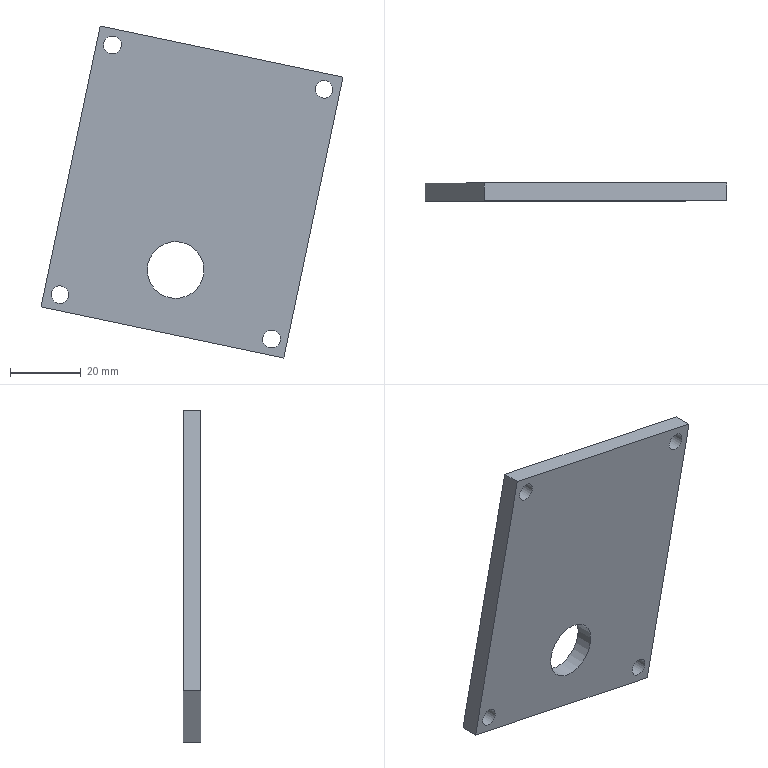Part | STEP file | 2_ESTAGIO_006-01 | 1 solid | 11 faces | box 85.161 x 5 x 93.664 mm | volume 26952 mm3 | plane 6 | cylinder 5 | commonest cylinder face diameters 5 x4 16 x1
STEP:
#1=CARTESIAN_POINT('',(0.,0.,0.));
#2=DIRECTION('',(0.,0.,1.));
#3=DIRECTION('',(1.,0.,0.));
#4=AXIS2_PLACEMENT_3D('',#1,#2,#3);
#5=CARTESIAN_POINT('',(432.411,-532.65,430.025));
#6=VERTEX_POINT('',#5);
#7=CARTESIAN_POINT('',(430.217,-532.65,428.827));
#8=DIRECTION('',(0.,-1.,0.));
#9=DIRECTION('',(1.,0.,0.));
#10=AXIS2_PLACEMENT_3D('',#7,#8,#9);
#11=CIRCLE('',#10,2.5);
#12=CARTESIAN_POINT('',(430.217,-532.75,428.827));
#13=DIRECTION('',(0.,-1.,0.));
#14=DIRECTION('',(0.8776,0.,0.4794));
#15=AXIS2_PLACEMENT_3D('',#12,#13,#14);
#16=CYLINDRICAL_SURFACE('',#15,2.5);
#17=CARTESIAN_POINT('',(-0.5,-0.1));
#18=DIRECTION('',(1.,0.));
#19=VECTOR('',#18,1.);
#20=LINE('',#17,#19);
#21=(GEOMETRIC_REPRESENTATION_CONTEXT(2)PARAMETRIC_REPRESENTATION_CONTEXT()REPRESENTATION_CONTEXT('',''));
#22=DEFINITIONAL_REPRESENTATION('',(#20),#21);
#23=PCURVE('',#16,#22);
#24=CARTESIAN_POINT('',(435.546,-532.65,432.305));
#25=DIRECTION('',(0.,1.,0.));
#26=DIRECTION('',(0.,0.,1.));
#27=AXIS2_PLACEMENT_3D('',#24,#25,#26);
#28=PLANE('',#27);
#29=CARTESIAN_POINT('',(-3.478,-2.829));
#30=CARTESIAN_POINT('',(0.8517,-2.829));
#31=CARTESIAN_POINT('',(-1.313,-6.579));
#32=CARTESIAN_POINT('',(-3.478,-10.329));
#33=CARTESIAN_POINT('',(-5.643,-6.579));
#34=CARTESIAN_POINT('',(-7.809,-2.829));
#35=CARTESIAN_POINT('',(-3.478,-2.829));
#36=(BOUNDED_CURVE()B_SPLINE_CURVE(2,(#29,#30,#31,#32,#33,#34,#35),.UNSPECIFIED.,.T.,.F.)B_SPLINE_CURVE_WITH_KNOTS((1,2,2,2,2,1),(-2.094,0.,2.094,4.189,6.283,8.378),.UNSPECIFIED.)CURVE()GEOMETRIC_REPRESENTATION_ITEM()RATIONAL_B_SPLINE_CURVE((1.,0.5,1.,0.5,1.,0.5,1.))REPRESENTATION_ITEM(''));
#37=(GEOMETRIC_REPRESENTATION_CONTEXT(2)PARAMETRIC_REPRESENTATION_CONTEXT()REPRESENTATION_CONTEXT('',''));
#38=DEFINITIONAL_REPRESENTATION('',(#36),#37);
#39=PCURVE('',#28,#38);
#40=SURFACE_CURVE('',#11,(#23,#39),.PCURVE_S1.);
#41=EDGE_CURVE('',#6,#6,#40,.T.);
#42=ORIENTED_EDGE('',*,*,#41,.T.);
#43=CARTESIAN_POINT('',(432.411,-537.65,430.025));
#44=VERTEX_POINT('',#43);
#45=CARTESIAN_POINT('',(432.411,-532.65,430.025));
#46=CARTESIAN_POINT('',(432.411,-537.65,430.025));
#47=B_SPLINE_CURVE_WITH_KNOTS('',1,(#45,#46),.UNSPECIFIED.,.F.,.F.,(2,2),(-0.1,4.9),.PIECEWISE_BEZIER_KNOTS.);
#48=CARTESIAN_POINT('',(6.283,0.));
#49=DIRECTION('',(0.,1.));
#50=VECTOR('',#49,1.);
#51=LINE('',#48,#50);
#52=(GEOMETRIC_REPRESENTATION_CONTEXT(2)PARAMETRIC_REPRESENTATION_CONTEXT()REPRESENTATION_CONTEXT('',''));
#53=DEFINITIONAL_REPRESENTATION('',(#51),#52);
#54=PCURVE('',#16,#53);
#55=CARTESIAN_POINT('',(0.,0.));
#56=DIRECTION('',(0.,1.));
#57=VECTOR('',#56,1.);
#58=LINE('',#55,#57);
#59=(GEOMETRIC_REPRESENTATION_CONTEXT(2)PARAMETRIC_REPRESENTATION_CONTEXT()REPRESENTATION_CONTEXT('',''));
#60=DEFINITIONAL_REPRESENTATION('',(#58),#59);
#61=PCURVE('',#16,#60);
#62=SEAM_CURVE('',#47,(#54,#61),.PCURVE_S1.);
#63=EDGE_CURVE('',#6,#44,#62,.T.);
#64=ORIENTED_EDGE('',*,*,#63,.T.);
#65=CARTESIAN_POINT('',(430.217,-537.65,428.827));
#66=DIRECTION('',(0.,-1.,0.));
#67=DIRECTION('',(1.,0.,0.));
#68=AXIS2_PLACEMENT_3D('',#65,#66,#67);
#69=CIRCLE('',#68,2.5);
#70=CARTESIAN_POINT('',(-0.5,4.9));
#71=DIRECTION('',(1.,0.));
#72=VECTOR('',#71,1.);
#73=LINE('',#70,#72);
#74=(GEOMETRIC_REPRESENTATION_CONTEXT(2)PARAMETRIC_REPRESENTATION_CONTEXT()REPRESENTATION_CONTEXT('',''));
#75=DEFINITIONAL_REPRESENTATION('',(#73),#74);
#76=PCURVE('',#16,#75);
#77=CARTESIAN_POINT('',(435.546,-537.65,432.305));
#78=DIRECTION('',(0.,1.,0.));
#79=DIRECTION('',(0.,0.,1.));
#80=AXIS2_PLACEMENT_3D('',#77,#78,#79);
#81=PLANE('',#80);
#82=CARTESIAN_POINT('',(-3.478,-2.829));
#83=CARTESIAN_POINT('',(0.8517,-2.829));
#84=CARTESIAN_POINT('',(-1.313,-6.579));
#85=CARTESIAN_POINT('',(-3.478,-10.329));
#86=CARTESIAN_POINT('',(-5.643,-6.579));
#87=CARTESIAN_POINT('',(-7.809,-2.829));
#88=CARTESIAN_POINT('',(-3.478,-2.829));
#89=(BOUNDED_CURVE()B_SPLINE_CURVE(2,(#82,#83,#84,#85,#86,#87,#88),.UNSPECIFIED.,.T.,.F.)B_SPLINE_CURVE_WITH_KNOTS((1,2,2,2,2,1),(-2.094,0.,2.094,4.189,6.283,8.378),.UNSPECIFIED.)CURVE()GEOMETRIC_REPRESENTATION_ITEM()RATIONAL_B_SPLINE_CURVE((1.,0.5,1.,0.5,1.,0.5,1.))REPRESENTATION_ITEM(''));
#90=(GEOMETRIC_REPRESENTATION_CONTEXT(2)PARAMETRIC_REPRESENTATION_CONTEXT()REPRESENTATION_CONTEXT('',''));
#91=DEFINITIONAL_REPRESENTATION('',(#89),#90);
#92=PCURVE('',#81,#91);
#93=SURFACE_CURVE('',#69,(#76,#92),.PCURVE_S1.);
#94=EDGE_CURVE('',#44,#44,#93,.T.);
#95=ORIENTED_EDGE('',*,*,#94,.F.);
#96=ORIENTED_EDGE('',*,*,#63,.F.);
#97=EDGE_LOOP('',(#42,#64,#95,#96));
#98=FACE_BOUND('',#97,.F.);
#99=ADVANCED_FACE('',(#98),#16,.F.);
#100=CARTESIAN_POINT('',(418.889,-537.65,353.036));
#101=VERTEX_POINT('',#100);
#102=CARTESIAN_POINT('',(418.889,-532.65,353.036));
#103=VERTEX_POINT('',#102);
#104=CARTESIAN_POINT('',(418.889,-537.65,353.036));
#105=DIRECTION('',(0.,1.,0.));
#106=VECTOR('',#105,1.);
#107=LINE('',#104,#106);
#108=CARTESIAN_POINT('',(418.889,-537.65,353.036));
#109=DIRECTION('',(-0.2056,0.,-0.9786));
#110=DIRECTION('',(-0.9786,0.,0.2056));
#111=AXIS2_PLACEMENT_3D('',#108,#109,#110);
#112=PLANE('',#111);
#113=CARTESIAN_POINT('',(0.,0.));
#114=DIRECTION('',(0.,1.));
#115=VECTOR('',#114,1.);
#116=LINE('',#113,#115);
#117=(GEOMETRIC_REPRESENTATION_CONTEXT(2)PARAMETRIC_REPRESENTATION_CONTEXT()REPRESENTATION_CONTEXT('',''));
#118=DEFINITIONAL_REPRESENTATION('',(#116),#117);
#119=PCURVE('',#112,#118);
#120=CARTESIAN_POINT('',(418.889,-537.65,353.036));
#121=DIRECTION('',(-0.9786,0.,0.2056));
#122=DIRECTION('',(0.2056,0.,0.9786));
#123=AXIS2_PLACEMENT_3D('',#120,#121,#122);
#124=PLANE('',#123);
#125=CARTESIAN_POINT('',(0.,0.));
#126=DIRECTION('',(0.,1.));
#127=VECTOR('',#126,1.);
#128=LINE('',#125,#127);
#129=(GEOMETRIC_REPRESENTATION_CONTEXT(2)PARAMETRIC_REPRESENTATION_CONTEXT()REPRESENTATION_CONTEXT('',''));
#130=DEFINITIONAL_REPRESENTATION('',(#128),#129);
#131=PCURVE('',#124,#130);
#132=SURFACE_CURVE('',#107,(#119,#131),.PCURVE_S1.);
#133=EDGE_CURVE('',#101,#103,#132,.T.);
#134=ORIENTED_EDGE('',*,*,#133,.F.);
#135=CARTESIAN_POINT('',(350.385,-537.65,367.431));
#136=VERTEX_POINT('',#135);
#137=CARTESIAN_POINT('',(418.889,-537.65,353.036));
#138=DIRECTION('',(-0.9786,0.,0.2056));
#139=VECTOR('',#138,1.);
#140=LINE('',#137,#139);
#141=CARTESIAN_POINT('',(0.,0.));
#142=DIRECTION('',(1.,0.));
#143=VECTOR('',#142,1.);
#144=LINE('',#141,#143);
#145=(GEOMETRIC_REPRESENTATION_CONTEXT(2)PARAMETRIC_REPRESENTATION_CONTEXT()REPRESENTATION_CONTEXT('',''));
#146=DEFINITIONAL_REPRESENTATION('',(#144),#145);
#147=PCURVE('',#112,#146);
#148=CARTESIAN_POINT('',(-79.269,-16.657));
#149=DIRECTION('',(0.2056,-0.9786));
#150=VECTOR('',#149,1.);
#151=LINE('',#148,#150);
#152=(GEOMETRIC_REPRESENTATION_CONTEXT(2)PARAMETRIC_REPRESENTATION_CONTEXT()REPRESENTATION_CONTEXT('',''));
#153=DEFINITIONAL_REPRESENTATION('',(#151),#152);
#154=PCURVE('',#81,#153);
#155=SURFACE_CURVE('',#140,(#147,#154),.PCURVE_S1.);
#156=EDGE_CURVE('',#101,#136,#155,.T.);
#157=ORIENTED_EDGE('',*,*,#156,.T.);
#158=CARTESIAN_POINT('',(350.385,-532.65,367.431));
#159=VERTEX_POINT('',#158);
#160=CARTESIAN_POINT('',(350.385,-537.65,367.431));
#161=DIRECTION('',(0.,1.,0.));
#162=VECTOR('',#161,1.);
#163=LINE('',#160,#162);
#164=CARTESIAN_POINT('',(70.,0.));
#165=DIRECTION('',(0.,1.));
#166=VECTOR('',#165,1.);
#167=LINE('',#164,#166);
#168=(GEOMETRIC_REPRESENTATION_CONTEXT(2)PARAMETRIC_REPRESENTATION_CONTEXT()REPRESENTATION_CONTEXT('',''));
#169=DEFINITIONAL_REPRESENTATION('',(#167),#168);
#170=PCURVE('',#112,#169);
#171=CARTESIAN_POINT('',(367.043,-537.65,446.7));
#172=DIRECTION('',(0.9786,0.,-0.2056));
#173=DIRECTION('',(-0.2056,0.,-0.9786));
#174=AXIS2_PLACEMENT_3D('',#171,#172,#173);
#175=PLANE('',#174);
#176=CARTESIAN_POINT('',(81.,0.));
#177=DIRECTION('',(0.,1.));
#178=VECTOR('',#177,1.);
#179=LINE('',#176,#178);
#180=(GEOMETRIC_REPRESENTATION_CONTEXT(2)PARAMETRIC_REPRESENTATION_CONTEXT()REPRESENTATION_CONTEXT('',''));
#181=DEFINITIONAL_REPRESENTATION('',(#179),#180);
#182=PCURVE('',#175,#181);
#183=SURFACE_CURVE('',#163,(#170,#182),.PCURVE_S1.);
#184=EDGE_CURVE('',#136,#159,#183,.T.);
#185=ORIENTED_EDGE('',*,*,#184,.T.);
#186=CARTESIAN_POINT('',(418.889,-532.65,353.036));
#187=DIRECTION('',(-0.9786,0.,0.2056));
#188=VECTOR('',#187,1.);
#189=LINE('',#186,#188);
#190=CARTESIAN_POINT('',(0.,5.));
#191=DIRECTION('',(1.,0.));
#192=VECTOR('',#191,1.);
#193=LINE('',#190,#192);
#194=(GEOMETRIC_REPRESENTATION_CONTEXT(2)PARAMETRIC_REPRESENTATION_CONTEXT()REPRESENTATION_CONTEXT('',''));
#195=DEFINITIONAL_REPRESENTATION('',(#193),#194);
#196=PCURVE('',#112,#195);
#197=CARTESIAN_POINT('',(-79.269,-16.657));
#198=DIRECTION('',(0.2056,-0.9786));
#199=VECTOR('',#198,1.);
#200=LINE('',#197,#199);
#201=(GEOMETRIC_REPRESENTATION_CONTEXT(2)PARAMETRIC_REPRESENTATION_CONTEXT()REPRESENTATION_CONTEXT('',''));
#202=DEFINITIONAL_REPRESENTATION('',(#200),#201);
#203=PCURVE('',#28,#202);
#204=SURFACE_CURVE('',#189,(#196,#203),.PCURVE_S1.);
#205=EDGE_CURVE('',#103,#159,#204,.T.);
#206=ORIENTED_EDGE('',*,*,#205,.F.);
#207=EDGE_LOOP('',(#134,#157,#185,#206));
#208=FACE_BOUND('',#207,.T.);
#209=ADVANCED_FACE('',(#208),#112,.T.);
#210=ORIENTED_EDGE('',*,*,#184,.F.);
#211=CARTESIAN_POINT('',(367.043,-537.65,446.7));
#212=VERTEX_POINT('',#211);
#213=CARTESIAN_POINT('',(367.043,-537.65,446.7));
#214=DIRECTION('',(-0.2056,0.,-0.9786));
#215=VECTOR('',#214,1.);
#216=LINE('',#213,#215);
#217=CARTESIAN_POINT('',(0.,0.));
#218=DIRECTION('',(1.,0.));
#219=VECTOR('',#218,1.);
#220=LINE('',#217,#219);
#221=(GEOMETRIC_REPRESENTATION_CONTEXT(2)PARAMETRIC_REPRESENTATION_CONTEXT()REPRESENTATION_CONTEXT('',''));
#222=DEFINITIONAL_REPRESENTATION('',(#220),#221);
#223=PCURVE('',#175,#222);
#224=CARTESIAN_POINT('',(14.395,-68.504));
#225=DIRECTION('',(-0.9786,-0.2056));
#226=VECTOR('',#225,1.);
#227=LINE('',#224,#226);
#228=(GEOMETRIC_REPRESENTATION_CONTEXT(2)PARAMETRIC_REPRESENTATION_CONTEXT()REPRESENTATION_CONTEXT('',''));
#229=DEFINITIONAL_REPRESENTATION('',(#227),#228);
#230=PCURVE('',#81,#229);
#231=SURFACE_CURVE('',#216,(#223,#230),.PCURVE_S1.);
#232=EDGE_CURVE('',#212,#136,#231,.T.);
#233=ORIENTED_EDGE('',*,*,#232,.F.);
#234=CARTESIAN_POINT('',(367.043,-532.65,446.7));
#235=VERTEX_POINT('',#234);
#236=CARTESIAN_POINT('',(367.043,-537.65,446.7));
#237=DIRECTION('',(0.,1.,0.));
#238=VECTOR('',#237,1.);
#239=LINE('',#236,#238);
#240=CARTESIAN_POINT('',(0.,0.));
#241=DIRECTION('',(0.,1.));
#242=VECTOR('',#241,1.);
#243=LINE('',#240,#242);
#244=(GEOMETRIC_REPRESENTATION_CONTEXT(2)PARAMETRIC_REPRESENTATION_CONTEXT()REPRESENTATION_CONTEXT('',''));
#245=DEFINITIONAL_REPRESENTATION('',(#243),#244);
#246=PCURVE('',#175,#245);
#247=CARTESIAN_POINT('',(367.043,-537.65,446.7));
#248=DIRECTION('',(0.2056,0.,0.9786));
#249=DIRECTION('',(0.9786,0.,-0.2056));
#250=AXIS2_PLACEMENT_3D('',#247,#248,#249);
#251=PLANE('',#250);
#252=CARTESIAN_POINT('',(0.,0.));
#253=DIRECTION('',(0.,1.));
#254=VECTOR('',#253,1.);
#255=LINE('',#252,#254);
#256=(GEOMETRIC_REPRESENTATION_CONTEXT(2)PARAMETRIC_REPRESENTATION_CONTEXT()REPRESENTATION_CONTEXT('',''));
#257=DEFINITIONAL_REPRESENTATION('',(#255),#256);
#258=PCURVE('',#251,#257);
#259=SURFACE_CURVE('',#239,(#246,#258),.PCURVE_S1.);
#260=EDGE_CURVE('',#212,#235,#259,.T.);
#261=ORIENTED_EDGE('',*,*,#260,.T.);
#262=CARTESIAN_POINT('',(367.043,-532.65,446.7));
#263=DIRECTION('',(-0.2056,0.,-0.9786));
#264=VECTOR('',#263,1.);
#265=LINE('',#262,#264);
#266=CARTESIAN_POINT('',(0.,5.));
#267=DIRECTION('',(1.,0.));
#268=VECTOR('',#267,1.);
#269=LINE('',#266,#268);
#270=(GEOMETRIC_REPRESENTATION_CONTEXT(2)PARAMETRIC_REPRESENTATION_CONTEXT()REPRESENTATION_CONTEXT('',''));
#271=DEFINITIONAL_REPRESENTATION('',(#269),#270);
#272=PCURVE('',#175,#271);
#273=CARTESIAN_POINT('',(14.395,-68.504));
#274=DIRECTION('',(-0.9786,-0.2056));
#275=VECTOR('',#274,1.);
#276=LINE('',#273,#275);
#277=(GEOMETRIC_REPRESENTATION_CONTEXT(2)PARAMETRIC_REPRESENTATION_CONTEXT()REPRESENTATION_CONTEXT('',''));
#278=DEFINITIONAL_REPRESENTATION('',(#276),#277);
#279=PCURVE('',#28,#278);
#280=SURFACE_CURVE('',#265,(#272,#279),.PCURVE_S1.);
#281=EDGE_CURVE('',#235,#159,#280,.T.);
#282=ORIENTED_EDGE('',*,*,#281,.T.);
#283=EDGE_LOOP('',(#210,#233,#261,#282));
#284=FACE_BOUND('',#283,.T.);
#285=ADVANCED_FACE('',(#284),#175,.F.);
#286=ORIENTED_EDGE('',*,*,#260,.F.);
#287=CARTESIAN_POINT('',(435.546,-537.65,432.305));
#288=VERTEX_POINT('',#287);
#289=CARTESIAN_POINT('',(367.043,-537.65,446.7));
#290=DIRECTION('',(0.9786,0.,-0.2056));
#291=VECTOR('',#290,1.);
#292=LINE('',#289,#291);
#293=CARTESIAN_POINT('',(0.,0.));
#294=DIRECTION('',(1.,0.));
#295=VECTOR('',#294,1.);
#296=LINE('',#293,#295);
#297=(GEOMETRIC_REPRESENTATION_CONTEXT(2)PARAMETRIC_REPRESENTATION_CONTEXT()REPRESENTATION_CONTEXT('',''));
#298=DEFINITIONAL_REPRESENTATION('',(#296),#297);
#299=PCURVE('',#251,#298);
#300=CARTESIAN_POINT('',(14.395,-68.504));
#301=DIRECTION('',(-0.2056,0.9786));
#302=VECTOR('',#301,1.);
#303=LINE('',#300,#302);
#304=(GEOMETRIC_REPRESENTATION_CONTEXT(2)PARAMETRIC_REPRESENTATION_CONTEXT()REPRESENTATION_CONTEXT('',''));
#305=DEFINITIONAL_REPRESENTATION('',(#303),#304);
#306=PCURVE('',#81,#305);
#307=SURFACE_CURVE('',#292,(#299,#306),.PCURVE_S1.);
#308=EDGE_CURVE('',#212,#288,#307,.T.);
#309=ORIENTED_EDGE('',*,*,#308,.T.);
#310=CARTESIAN_POINT('',(435.546,-532.65,432.305));
#311=VERTEX_POINT('',#310);
#312=CARTESIAN_POINT('',(435.546,-537.65,432.305));
#313=DIRECTION('',(0.,1.,0.));
#314=VECTOR('',#313,1.);
#315=LINE('',#312,#314);
#316=CARTESIAN_POINT('',(70.,0.));
#317=DIRECTION('',(0.,1.));
#318=VECTOR('',#317,1.);
#319=LINE('',#316,#318);
#320=(GEOMETRIC_REPRESENTATION_CONTEXT(2)PARAMETRIC_REPRESENTATION_CONTEXT()REPRESENTATION_CONTEXT('',''));
#321=DEFINITIONAL_REPRESENTATION('',(#319),#320);
#322=PCURVE('',#251,#321);
#323=CARTESIAN_POINT('',(81.,0.));
#324=DIRECTION('',(0.,1.));
#325=VECTOR('',#324,1.);
#326=LINE('',#323,#325);
#327=(GEOMETRIC_REPRESENTATION_CONTEXT(2)PARAMETRIC_REPRESENTATION_CONTEXT()REPRESENTATION_CONTEXT('',''));
#328=DEFINITIONAL_REPRESENTATION('',(#326),#327);
#329=PCURVE('',#124,#328);
#330=SURFACE_CURVE('',#315,(#322,#329),.PCURVE_S1.);
#331=EDGE_CURVE('',#288,#311,#330,.T.);
#332=ORIENTED_EDGE('',*,*,#331,.T.);
#333=CARTESIAN_POINT('',(367.043,-532.65,446.7));
#334=DIRECTION('',(0.9786,0.,-0.2056));
#335=VECTOR('',#334,1.);
#336=LINE('',#333,#335);
#337=CARTESIAN_POINT('',(0.,5.));
#338=DIRECTION('',(1.,0.));
#339=VECTOR('',#338,1.);
#340=LINE('',#337,#339);
#341=(GEOMETRIC_REPRESENTATION_CONTEXT(2)PARAMETRIC_REPRESENTATION_CONTEXT()REPRESENTATION_CONTEXT('',''));
#342=DEFINITIONAL_REPRESENTATION('',(#340),#341);
#343=PCURVE('',#251,#342);
#344=CARTESIAN_POINT('',(14.395,-68.504));
#345=DIRECTION('',(-0.2056,0.9786));
#346=VECTOR('',#345,1.);
#347=LINE('',#344,#346);
#348=(GEOMETRIC_REPRESENTATION_CONTEXT(2)PARAMETRIC_REPRESENTATION_CONTEXT()REPRESENTATION_CONTEXT('',''));
#349=DEFINITIONAL_REPRESENTATION('',(#347),#348);
#350=PCURVE('',#28,#349);
#351=SURFACE_CURVE('',#336,(#343,#350),.PCURVE_S1.);
#352=EDGE_CURVE('',#235,#311,#351,.T.);
#353=ORIENTED_EDGE('',*,*,#352,.F.);
#354=EDGE_LOOP('',(#286,#309,#332,#353));
#355=FACE_BOUND('',#354,.T.);
#356=ADVANCED_FACE('',(#355),#251,.T.);
#357=ORIENTED_EDGE('',*,*,#331,.F.);
#358=CARTESIAN_POINT('',(418.889,-537.65,353.036));
#359=DIRECTION('',(0.2056,0.,0.9786));
#360=VECTOR('',#359,1.);
#361=LINE('',#358,#360);
#362=CARTESIAN_POINT('',(0.,0.));
#363=DIRECTION('',(1.,0.));
#364=VECTOR('',#363,1.);
#365=LINE('',#362,#364);
#366=(GEOMETRIC_REPRESENTATION_CONTEXT(2)PARAMETRIC_REPRESENTATION_CONTEXT()REPRESENTATION_CONTEXT('',''));
#367=DEFINITIONAL_REPRESENTATION('',(#365),#366);
#368=PCURVE('',#124,#367);
#369=CARTESIAN_POINT('',(-79.269,-16.657));
#370=DIRECTION('',(0.9786,0.2056));
#371=VECTOR('',#370,1.);
#372=LINE('',#369,#371);
#373=(GEOMETRIC_REPRESENTATION_CONTEXT(2)PARAMETRIC_REPRESENTATION_CONTEXT()REPRESENTATION_CONTEXT('',''));
#374=DEFINITIONAL_REPRESENTATION('',(#372),#373);
#375=PCURVE('',#81,#374);
#376=SURFACE_CURVE('',#361,(#368,#375),.PCURVE_S1.);
#377=EDGE_CURVE('',#101,#288,#376,.T.);
#378=ORIENTED_EDGE('',*,*,#377,.F.);
#379=ORIENTED_EDGE('',*,*,#133,.T.);
#380=CARTESIAN_POINT('',(418.889,-532.65,353.036));
#381=DIRECTION('',(0.2056,0.,0.9786));
#382=VECTOR('',#381,1.);
#383=LINE('',#380,#382);
#384=CARTESIAN_POINT('',(0.,5.));
#385=DIRECTION('',(1.,0.));
#386=VECTOR('',#385,1.);
#387=LINE('',#384,#386);
#388=(GEOMETRIC_REPRESENTATION_CONTEXT(2)PARAMETRIC_REPRESENTATION_CONTEXT()REPRESENTATION_CONTEXT('',''));
#389=DEFINITIONAL_REPRESENTATION('',(#387),#388);
#390=PCURVE('',#124,#389);
#391=CARTESIAN_POINT('',(-79.269,-16.657));
#392=DIRECTION('',(0.9786,0.2056));
#393=VECTOR('',#392,1.);
#394=LINE('',#391,#393);
#395=(GEOMETRIC_REPRESENTATION_CONTEXT(2)PARAMETRIC_REPRESENTATION_CONTEXT()REPRESENTATION_CONTEXT('',''));
#396=DEFINITIONAL_REPRESENTATION('',(#394),#395);
#397=PCURVE('',#28,#396);
#398=SURFACE_CURVE('',#383,(#390,#397),.PCURVE_S1.);
#399=EDGE_CURVE('',#103,#311,#398,.T.);
#400=ORIENTED_EDGE('',*,*,#399,.T.);
#401=EDGE_LOOP('',(#357,#378,#379,#400));
#402=FACE_BOUND('',#401,.T.);
#403=ADVANCED_FACE('',(#402),#124,.F.);
#404=CARTESIAN_POINT('',(395.36,-532.65,381.685));
#405=VERTEX_POINT('',#404);
#406=CARTESIAN_POINT('',(388.339,-532.65,377.849));
#407=DIRECTION('',(0.,-1.,0.));
#408=DIRECTION('',(1.,0.,0.));
#409=AXIS2_PLACEMENT_3D('',#406,#407,#408);
#410=CIRCLE('',#409,8.);
#411=CARTESIAN_POINT('',(388.339,-532.75,377.849));
#412=DIRECTION('',(0.,-1.,0.));
#413=DIRECTION('',(0.8776,0.,0.4794));
#414=AXIS2_PLACEMENT_3D('',#411,#412,#413);
#415=CYLINDRICAL_SURFACE('',#414,8.);
#416=CARTESIAN_POINT('',(-0.5,-0.1));
#417=DIRECTION('',(1.,0.));
#418=VECTOR('',#417,1.);
#419=LINE('',#416,#418);
#420=(GEOMETRIC_REPRESENTATION_CONTEXT(2)PARAMETRIC_REPRESENTATION_CONTEXT()REPRESENTATION_CONTEXT('',''));
#421=DEFINITIONAL_REPRESENTATION('',(#419),#420);
#422=PCURVE('',#415,#421);
#423=CARTESIAN_POINT('',(-54.456,-39.207));
#424=CARTESIAN_POINT('',(-40.6,-39.207));
#425=CARTESIAN_POINT('',(-47.528,-51.207));
#426=CARTESIAN_POINT('',(-54.456,-63.207));
#427=CARTESIAN_POINT('',(-61.384,-51.207));
#428=CARTESIAN_POINT('',(-68.312,-39.207));
#429=CARTESIAN_POINT('',(-54.456,-39.207));
#430=(BOUNDED_CURVE()B_SPLINE_CURVE(2,(#423,#424,#425,#426,#427,#428,#429),.UNSPECIFIED.,.T.,.F.)B_SPLINE_CURVE_WITH_KNOTS((1,2,2,2,2,1),(-2.094,0.,2.094,4.189,6.283,8.378),.UNSPECIFIED.)CURVE()GEOMETRIC_REPRESENTATION_ITEM()RATIONAL_B_SPLINE_CURVE((1.,0.5,1.,0.5,1.,0.5,1.))REPRESENTATION_ITEM(''));
#431=(GEOMETRIC_REPRESENTATION_CONTEXT(2)PARAMETRIC_REPRESENTATION_CONTEXT()REPRESENTATION_CONTEXT('',''));
#432=DEFINITIONAL_REPRESENTATION('',(#430),#431);
#433=PCURVE('',#28,#432);
#434=SURFACE_CURVE('',#410,(#422,#433),.PCURVE_S1.);
#435=EDGE_CURVE('',#405,#405,#434,.T.);
#436=ORIENTED_EDGE('',*,*,#435,.T.);
#437=CARTESIAN_POINT('',(395.36,-537.65,381.685));
#438=VERTEX_POINT('',#437);
#439=CARTESIAN_POINT('',(395.36,-532.65,381.685));
#440=CARTESIAN_POINT('',(395.36,-537.65,381.685));
#441=B_SPLINE_CURVE_WITH_KNOTS('',1,(#439,#440),.UNSPECIFIED.,.F.,.F.,(2,2),(-0.1,4.9),.PIECEWISE_BEZIER_KNOTS.);
#442=CARTESIAN_POINT('',(6.283,0.));
#443=DIRECTION('',(0.,1.));
#444=VECTOR('',#443,1.);
#445=LINE('',#442,#444);
#446=(GEOMETRIC_REPRESENTATION_CONTEXT(2)PARAMETRIC_REPRESENTATION_CONTEXT()REPRESENTATION_CONTEXT('',''));
#447=DEFINITIONAL_REPRESENTATION('',(#445),#446);
#448=PCURVE('',#415,#447);
#449=CARTESIAN_POINT('',(0.,0.));
#450=DIRECTION('',(0.,1.));
#451=VECTOR('',#450,1.);
#452=LINE('',#449,#451);
#453=(GEOMETRIC_REPRESENTATION_CONTEXT(2)PARAMETRIC_REPRESENTATION_CONTEXT()REPRESENTATION_CONTEXT('',''));
#454=DEFINITIONAL_REPRESENTATION('',(#452),#453);
#455=PCURVE('',#415,#454);
#456=SEAM_CURVE('',#441,(#448,#455),.PCURVE_S1.);
#457=EDGE_CURVE('',#405,#438,#456,.T.);
#458=ORIENTED_EDGE('',*,*,#457,.T.);
#459=CARTESIAN_POINT('',(388.339,-537.65,377.849));
#460=DIRECTION('',(0.,-1.,0.));
#461=DIRECTION('',(1.,0.,0.));
#462=AXIS2_PLACEMENT_3D('',#459,#460,#461);
#463=CIRCLE('',#462,8.);
#464=CARTESIAN_POINT('',(-0.5,4.9));
#465=DIRECTION('',(1.,0.));
#466=VECTOR('',#465,1.);
#467=LINE('',#464,#466);
#468=(GEOMETRIC_REPRESENTATION_CONTEXT(2)PARAMETRIC_REPRESENTATION_CONTEXT()REPRESENTATION_CONTEXT('',''));
#469=DEFINITIONAL_REPRESENTATION('',(#467),#468);
#470=PCURVE('',#415,#469);
#471=CARTESIAN_POINT('',(-54.456,-39.207));
#472=CARTESIAN_POINT('',(-40.6,-39.207));
#473=CARTESIAN_POINT('',(-47.528,-51.207));
#474=CARTESIAN_POINT('',(-54.456,-63.207));
#475=CARTESIAN_POINT('',(-61.384,-51.207));
#476=CARTESIAN_POINT('',(-68.312,-39.207));
#477=CARTESIAN_POINT('',(-54.456,-39.207));
#478=(BOUNDED_CURVE()B_SPLINE_CURVE(2,(#471,#472,#473,#474,#475,#476,#477),.UNSPECIFIED.,.T.,.F.)B_SPLINE_CURVE_WITH_KNOTS((1,2,2,2,2,1),(-2.094,0.,2.094,4.189,6.283,8.378),.UNSPECIFIED.)CURVE()GEOMETRIC_REPRESENTATION_ITEM()RATIONAL_B_SPLINE_CURVE((1.,0.5,1.,0.5,1.,0.5,1.))REPRESENTATION_ITEM(''));
#479=(GEOMETRIC_REPRESENTATION_CONTEXT(2)PARAMETRIC_REPRESENTATION_CONTEXT()REPRESENTATION_CONTEXT('',''));
#480=DEFINITIONAL_REPRESENTATION('',(#478),#479);
#481=PCURVE('',#81,#480);
#482=SURFACE_CURVE('',#463,(#470,#481),.PCURVE_S1.);
#483=EDGE_CURVE('',#438,#438,#482,.T.);
#484=ORIENTED_EDGE('',*,*,#483,.F.);
#485=ORIENTED_EDGE('',*,*,#457,.F.);
#486=EDGE_LOOP('',(#436,#458,#484,#485));
#487=FACE_BOUND('',#486,.F.);
#488=ADVANCED_FACE('',(#487),#415,.F.);
#489=ORIENTED_EDGE('',*,*,#377,.T.);
#490=ORIENTED_EDGE('',*,*,#308,.F.);
#491=ORIENTED_EDGE('',*,*,#232,.T.);
#492=ORIENTED_EDGE('',*,*,#156,.F.);
#493=EDGE_LOOP('',(#489,#490,#491,#492));
#494=FACE_BOUND('',#493,.T.);
#495=ORIENTED_EDGE('',*,*,#94,.F.);
#496=EDGE_LOOP('',(#495));
#497=FACE_BOUND('',#496,.T.);
#498=ORIENTED_EDGE('',*,*,#483,.F.);
#499=EDGE_LOOP('',(#498));
#500=FACE_BOUND('',#499,.T.);
#501=CARTESIAN_POINT('',(417.605,-537.65,359.564));
#502=VERTEX_POINT('',#501);
#503=CARTESIAN_POINT('',(415.411,-537.65,358.366));
#504=DIRECTION('',(0.,1.,0.));
#505=DIRECTION('',(1.,0.,0.));
#506=AXIS2_PLACEMENT_3D('',#503,#504,#505);
#507=CIRCLE('',#506,2.5);
#508=CARTESIAN_POINT('',(-73.94,-20.136));
#509=DIRECTION('',(0.,1.));
#510=AXIS2_PLACEMENT_2D('',#508,#509);
#511=CIRCLE('',#510,2.5);
#512=(GEOMETRIC_REPRESENTATION_CONTEXT(2)PARAMETRIC_REPRESENTATION_CONTEXT()REPRESENTATION_CONTEXT('',''));
#513=DEFINITIONAL_REPRESENTATION('',(#511),#512);
#514=PCURVE('',#81,#513);
#515=CARTESIAN_POINT('',(415.411,-532.75,358.366));
#516=DIRECTION('',(0.,-1.,0.));
#517=DIRECTION('',(0.8776,0.,0.4794));
#518=AXIS2_PLACEMENT_3D('',#515,#516,#517);
#519=CYLINDRICAL_SURFACE('',#518,2.5);
#520=CARTESIAN_POINT('',(12.066,4.9));
#521=DIRECTION('',(-1.,0.));
#522=VECTOR('',#521,1.);
#523=LINE('',#520,#522);
#524=(GEOMETRIC_REPRESENTATION_CONTEXT(2)PARAMETRIC_REPRESENTATION_CONTEXT()REPRESENTATION_CONTEXT('',''));
#525=DEFINITIONAL_REPRESENTATION('',(#523),#524);
#526=PCURVE('',#519,#525);
#527=SURFACE_CURVE('',#507,(#514,#526),.PCURVE_S1.);
#528=EDGE_CURVE('',#502,#502,#527,.T.);
#529=ORIENTED_EDGE('',*,*,#528,.T.);
#530=EDGE_LOOP('',(#529));
#531=FACE_BOUND('',#530,.T.);
#532=CARTESIAN_POINT('',(372.715,-537.65,442.57));
#533=VERTEX_POINT('',#532);
#534=CARTESIAN_POINT('',(370.521,-537.65,441.371));
#535=DIRECTION('',(0.,1.,0.));
#536=DIRECTION('',(1.,0.,0.));
#537=AXIS2_PLACEMENT_3D('',#534,#535,#536);
#538=CIRCLE('',#537,2.5);
#539=CARTESIAN_POINT('',(9.066,-65.025));
#540=DIRECTION('',(0.,1.));
#541=AXIS2_PLACEMENT_2D('',#539,#540);
#542=CIRCLE('',#541,2.5);
#543=(GEOMETRIC_REPRESENTATION_CONTEXT(2)PARAMETRIC_REPRESENTATION_CONTEXT()REPRESENTATION_CONTEXT('',''));
#544=DEFINITIONAL_REPRESENTATION('',(#542),#543);
#545=PCURVE('',#81,#544);
#546=CARTESIAN_POINT('',(370.521,-532.75,441.371));
#547=DIRECTION('',(0.,-1.,0.));
#548=DIRECTION('',(0.8776,0.,0.4794));
#549=AXIS2_PLACEMENT_3D('',#546,#547,#548);
#550=CYLINDRICAL_SURFACE('',#549,2.5);
#551=CARTESIAN_POINT('',(12.066,4.9));
#552=DIRECTION('',(-1.,0.));
#553=VECTOR('',#552,1.);
#554=LINE('',#551,#553);
#555=(GEOMETRIC_REPRESENTATION_CONTEXT(2)PARAMETRIC_REPRESENTATION_CONTEXT()REPRESENTATION_CONTEXT('',''));
#556=DEFINITIONAL_REPRESENTATION('',(#554),#555);
#557=PCURVE('',#550,#556);
#558=SURFACE_CURVE('',#538,(#545,#557),.PCURVE_S1.);
#559=EDGE_CURVE('',#533,#533,#558,.T.);
#560=ORIENTED_EDGE('',*,*,#559,.T.);
#561=EDGE_LOOP('',(#560));
#562=FACE_BOUND('',#561,.T.);
#563=CARTESIAN_POINT('',(357.909,-537.65,372.108));
#564=VERTEX_POINT('',#563);
#565=CARTESIAN_POINT('',(355.715,-537.65,370.91));
#566=DIRECTION('',(0.,1.,0.));
#567=DIRECTION('',(1.,0.,0.));
#568=AXIS2_PLACEMENT_3D('',#565,#566,#567);
#569=CIRCLE('',#568,2.5);
#570=CARTESIAN_POINT('',(-61.395,-79.832));
#571=DIRECTION('',(0.,1.));
#572=AXIS2_PLACEMENT_2D('',#570,#571);
#573=CIRCLE('',#572,2.5);
#574=(GEOMETRIC_REPRESENTATION_CONTEXT(2)PARAMETRIC_REPRESENTATION_CONTEXT()REPRESENTATION_CONTEXT('',''));
#575=DEFINITIONAL_REPRESENTATION('',(#573),#574);
#576=PCURVE('',#81,#575);
#577=CARTESIAN_POINT('',(355.715,-532.75,370.91));
#578=DIRECTION('',(0.,-1.,0.));
#579=DIRECTION('',(0.8776,0.,0.4794));
#580=AXIS2_PLACEMENT_3D('',#577,#578,#579);
#581=CYLINDRICAL_SURFACE('',#580,2.5);
#582=CARTESIAN_POINT('',(12.066,4.9));
#583=DIRECTION('',(-1.,0.));
#584=VECTOR('',#583,1.);
#585=LINE('',#582,#584);
#586=(GEOMETRIC_REPRESENTATION_CONTEXT(2)PARAMETRIC_REPRESENTATION_CONTEXT()REPRESENTATION_CONTEXT('',''));
#587=DEFINITIONAL_REPRESENTATION('',(#585),#586);
#588=PCURVE('',#581,#587);
#589=SURFACE_CURVE('',#569,(#576,#588),.PCURVE_S1.);
#590=EDGE_CURVE('',#564,#564,#589,.T.);
#591=ORIENTED_EDGE('',*,*,#590,.T.);
#592=EDGE_LOOP('',(#591));
#593=FACE_BOUND('',#592,.T.);
#594=ADVANCED_FACE('',(#494,#497,#500,#531,#562,#593),#81,.F.);
#595=ORIENTED_EDGE('',*,*,#205,.T.);
#596=ORIENTED_EDGE('',*,*,#281,.F.);
#597=ORIENTED_EDGE('',*,*,#352,.T.);
#598=ORIENTED_EDGE('',*,*,#399,.F.);
#599=EDGE_LOOP('',(#595,#596,#597,#598));
#600=FACE_BOUND('',#599,.T.);
#601=ORIENTED_EDGE('',*,*,#41,.T.);
#602=EDGE_LOOP('',(#601));
#603=FACE_BOUND('',#602,.T.);
#604=ORIENTED_EDGE('',*,*,#435,.T.);
#605=EDGE_LOOP('',(#604));
#606=FACE_BOUND('',#605,.T.);
#607=CARTESIAN_POINT('',(417.605,-532.65,359.564));
#608=VERTEX_POINT('',#607);
#609=CARTESIAN_POINT('',(415.411,-532.65,358.366));
#610=DIRECTION('',(0.,1.,0.));
#611=DIRECTION('',(1.,0.,0.));
#612=AXIS2_PLACEMENT_3D('',#609,#610,#611);
#613=CIRCLE('',#612,2.5);
#614=CARTESIAN_POINT('',(-73.94,-20.136));
#615=DIRECTION('',(0.,1.));
#616=AXIS2_PLACEMENT_2D('',#614,#615);
#617=CIRCLE('',#616,2.5);
#618=(GEOMETRIC_REPRESENTATION_CONTEXT(2)PARAMETRIC_REPRESENTATION_CONTEXT()REPRESENTATION_CONTEXT('',''));
#619=DEFINITIONAL_REPRESENTATION('',(#617),#618);
#620=PCURVE('',#28,#619);
#621=CARTESIAN_POINT('',(12.066,-0.1));
#622=DIRECTION('',(-1.,0.));
#623=VECTOR('',#622,1.);
#624=LINE('',#621,#623);
#625=(GEOMETRIC_REPRESENTATION_CONTEXT(2)PARAMETRIC_REPRESENTATION_CONTEXT()REPRESENTATION_CONTEXT('',''));
#626=DEFINITIONAL_REPRESENTATION('',(#624),#625);
#627=PCURVE('',#519,#626);
#628=SURFACE_CURVE('',#613,(#620,#627),.PCURVE_S1.);
#629=EDGE_CURVE('',#608,#608,#628,.T.);
#630=ORIENTED_EDGE('',*,*,#629,.F.);
#631=EDGE_LOOP('',(#630));
#632=FACE_BOUND('',#631,.T.);
#633=CARTESIAN_POINT('',(372.715,-532.65,442.57));
#634=VERTEX_POINT('',#633);
#635=CARTESIAN_POINT('',(370.521,-532.65,441.371));
#636=DIRECTION('',(0.,1.,0.));
#637=DIRECTION('',(1.,0.,0.));
#638=AXIS2_PLACEMENT_3D('',#635,#636,#637);
#639=CIRCLE('',#638,2.5);
#640=CARTESIAN_POINT('',(9.066,-65.025));
#641=DIRECTION('',(0.,1.));
#642=AXIS2_PLACEMENT_2D('',#640,#641);
#643=CIRCLE('',#642,2.5);
#644=(GEOMETRIC_REPRESENTATION_CONTEXT(2)PARAMETRIC_REPRESENTATION_CONTEXT()REPRESENTATION_CONTEXT('',''));
#645=DEFINITIONAL_REPRESENTATION('',(#643),#644);
#646=PCURVE('',#28,#645);
#647=CARTESIAN_POINT('',(12.066,-0.1));
#648=DIRECTION('',(-1.,0.));
#649=VECTOR('',#648,1.);
#650=LINE('',#647,#649);
#651=(GEOMETRIC_REPRESENTATION_CONTEXT(2)PARAMETRIC_REPRESENTATION_CONTEXT()REPRESENTATION_CONTEXT('',''));
#652=DEFINITIONAL_REPRESENTATION('',(#650),#651);
#653=PCURVE('',#550,#652);
#654=SURFACE_CURVE('',#639,(#646,#653),.PCURVE_S1.);
#655=EDGE_CURVE('',#634,#634,#654,.T.);
#656=ORIENTED_EDGE('',*,*,#655,.F.);
#657=EDGE_LOOP('',(#656));
#658=FACE_BOUND('',#657,.T.);
#659=CARTESIAN_POINT('',(357.909,-532.65,372.108));
#660=VERTEX_POINT('',#659);
#661=CARTESIAN_POINT('',(355.715,-532.65,370.91));
#662=DIRECTION('',(0.,1.,0.));
#663=DIRECTION('',(1.,0.,0.));
#664=AXIS2_PLACEMENT_3D('',#661,#662,#663);
#665=CIRCLE('',#664,2.5);
#666=CARTESIAN_POINT('',(-61.395,-79.832));
#667=DIRECTION('',(0.,1.));
#668=AXIS2_PLACEMENT_2D('',#666,#667);
#669=CIRCLE('',#668,2.5);
#670=(GEOMETRIC_REPRESENTATION_CONTEXT(2)PARAMETRIC_REPRESENTATION_CONTEXT()REPRESENTATION_CONTEXT('',''));
#671=DEFINITIONAL_REPRESENTATION('',(#669),#670);
#672=PCURVE('',#28,#671);
#673=CARTESIAN_POINT('',(12.066,-0.1));
#674=DIRECTION('',(-1.,0.));
#675=VECTOR('',#674,1.);
#676=LINE('',#673,#675);
#677=(GEOMETRIC_REPRESENTATION_CONTEXT(2)PARAMETRIC_REPRESENTATION_CONTEXT()REPRESENTATION_CONTEXT('',''));
#678=DEFINITIONAL_REPRESENTATION('',(#676),#677);
#679=PCURVE('',#581,#678);
#680=SURFACE_CURVE('',#665,(#672,#679),.PCURVE_S1.);
#681=EDGE_CURVE('',#660,#660,#680,.T.);
#682=ORIENTED_EDGE('',*,*,#681,.F.);
#683=EDGE_LOOP('',(#682));
#684=FACE_BOUND('',#683,.T.);
#685=ADVANCED_FACE('',(#600,#603,#606,#632,#658,#684),#28,.T.);
#686=ORIENTED_EDGE('',*,*,#681,.F.);
#687=CARTESIAN_POINT('',(357.909,-532.65,372.108));
#688=CARTESIAN_POINT('',(357.909,-537.65,372.108));
#689=B_SPLINE_CURVE_WITH_KNOTS('',1,(#687,#688),.UNSPECIFIED.,.F.,.F.,(2,2),(-0.1,4.9),.PIECEWISE_BEZIER_KNOTS.);
#690=CARTESIAN_POINT('',(6.283,0.));
#691=DIRECTION('',(0.,1.));
#692=VECTOR('',#691,1.);
#693=LINE('',#690,#692);
#694=(GEOMETRIC_REPRESENTATION_CONTEXT(2)PARAMETRIC_REPRESENTATION_CONTEXT()REPRESENTATION_CONTEXT('',''));
#695=DEFINITIONAL_REPRESENTATION('',(#693),#694);
#696=PCURVE('',#581,#695);
#697=CARTESIAN_POINT('',(0.,0.));
#698=DIRECTION('',(0.,1.));
#699=VECTOR('',#698,1.);
#700=LINE('',#697,#699);
#701=(GEOMETRIC_REPRESENTATION_CONTEXT(2)PARAMETRIC_REPRESENTATION_CONTEXT()REPRESENTATION_CONTEXT('',''));
#702=DEFINITIONAL_REPRESENTATION('',(#700),#701);
#703=PCURVE('',#581,#702);
#704=SEAM_CURVE('',#689,(#696,#703),.PCURVE_S1.);
#705=EDGE_CURVE('',#660,#564,#704,.T.);
#706=ORIENTED_EDGE('',*,*,#705,.T.);
#707=ORIENTED_EDGE('',*,*,#590,.T.);
#708=ORIENTED_EDGE('',*,*,#705,.F.);
#709=EDGE_LOOP('',(#686,#706,#707,#708));
#710=FACE_BOUND('',#709,.F.);
#711=ADVANCED_FACE('',(#710),#581,.F.);
#712=ORIENTED_EDGE('',*,*,#655,.F.);
#713=CARTESIAN_POINT('',(372.715,-532.65,442.57));
#714=CARTESIAN_POINT('',(372.715,-537.65,442.57));
#715=B_SPLINE_CURVE_WITH_KNOTS('',1,(#713,#714),.UNSPECIFIED.,.F.,.F.,(2,2),(-0.1,4.9),.PIECEWISE_BEZIER_KNOTS.);
#716=CARTESIAN_POINT('',(6.283,0.));
#717=DIRECTION('',(0.,1.));
#718=VECTOR('',#717,1.);
#719=LINE('',#716,#718);
#720=(GEOMETRIC_REPRESENTATION_CONTEXT(2)PARAMETRIC_REPRESENTATION_CONTEXT()REPRESENTATION_CONTEXT('',''));
#721=DEFINITIONAL_REPRESENTATION('',(#719),#720);
#722=PCURVE('',#550,#721);
#723=CARTESIAN_POINT('',(0.,0.));
#724=DIRECTION('',(0.,1.));
#725=VECTOR('',#724,1.);
#726=LINE('',#723,#725);
#727=(GEOMETRIC_REPRESENTATION_CONTEXT(2)PARAMETRIC_REPRESENTATION_CONTEXT()REPRESENTATION_CONTEXT('',''));
#728=DEFINITIONAL_REPRESENTATION('',(#726),#727);
#729=PCURVE('',#550,#728);
#730=SEAM_CURVE('',#715,(#722,#729),.PCURVE_S1.);
#731=EDGE_CURVE('',#634,#533,#730,.T.);
#732=ORIENTED_EDGE('',*,*,#731,.T.);
#733=ORIENTED_EDGE('',*,*,#559,.T.);
#734=ORIENTED_EDGE('',*,*,#731,.F.);
#735=EDGE_LOOP('',(#712,#732,#733,#734));
#736=FACE_BOUND('',#735,.F.);
#737=ADVANCED_FACE('',(#736),#550,.F.);
#738=ORIENTED_EDGE('',*,*,#629,.F.);
#739=CARTESIAN_POINT('',(417.605,-532.65,359.564));
#740=CARTESIAN_POINT('',(417.605,-537.65,359.564));
#741=B_SPLINE_CURVE_WITH_KNOTS('',1,(#739,#740),.UNSPECIFIED.,.F.,.F.,(2,2),(-0.1,4.9),.PIECEWISE_BEZIER_KNOTS.);
#742=CARTESIAN_POINT('',(6.283,0.));
#743=DIRECTION('',(0.,1.));
#744=VECTOR('',#743,1.);
#745=LINE('',#742,#744);
#746=(GEOMETRIC_REPRESENTATION_CONTEXT(2)PARAMETRIC_REPRESENTATION_CONTEXT()REPRESENTATION_CONTEXT('',''));
#747=DEFINITIONAL_REPRESENTATION('',(#745),#746);
#748=PCURVE('',#519,#747);
#749=CARTESIAN_POINT('',(0.,0.));
#750=DIRECTION('',(0.,1.));
#751=VECTOR('',#750,1.);
#752=LINE('',#749,#751);
#753=(GEOMETRIC_REPRESENTATION_CONTEXT(2)PARAMETRIC_REPRESENTATION_CONTEXT()REPRESENTATION_CONTEXT('',''));
#754=DEFINITIONAL_REPRESENTATION('',(#752),#753);
#755=PCURVE('',#519,#754);
#756=SEAM_CURVE('',#741,(#748,#755),.PCURVE_S1.);
#757=EDGE_CURVE('',#608,#502,#756,.T.);
#758=ORIENTED_EDGE('',*,*,#757,.T.);
#759=ORIENTED_EDGE('',*,*,#528,.T.);
#760=ORIENTED_EDGE('',*,*,#757,.F.);
#761=EDGE_LOOP('',(#738,#758,#759,#760));
#762=FACE_BOUND('',#761,.F.);
#763=ADVANCED_FACE('',(#762),#519,.F.);
#764=CLOSED_SHELL('',(#99,#209,#285,#356,#403,#488,#594,#685,#711,#737,#763));
#765=MANIFOLD_SOLID_BREP('',#764);
#766=(LENGTH_UNIT()NAMED_UNIT(*)SI_UNIT(.MILLI.,.METRE.));
#767=UNCERTAINTY_MEASURE_WITH_UNIT(LENGTH_MEASURE(0.000005),#766,'','');
#768=(NAMED_UNIT(*)PLANE_ANGLE_UNIT()SI_UNIT($,.RADIAN.));
#769=(NAMED_UNIT(*)SI_UNIT($,.STERADIAN.)SOLID_ANGLE_UNIT());
#770=(GEOMETRIC_REPRESENTATION_CONTEXT(3)GLOBAL_UNCERTAINTY_ASSIGNED_CONTEXT((#767))GLOBAL_UNIT_ASSIGNED_CONTEXT((#766,#768,#769))REPRESENTATION_CONTEXT('',''));
#771=ADVANCED_BREP_SHAPE_REPRESENTATION('',(#4,#765),#770);